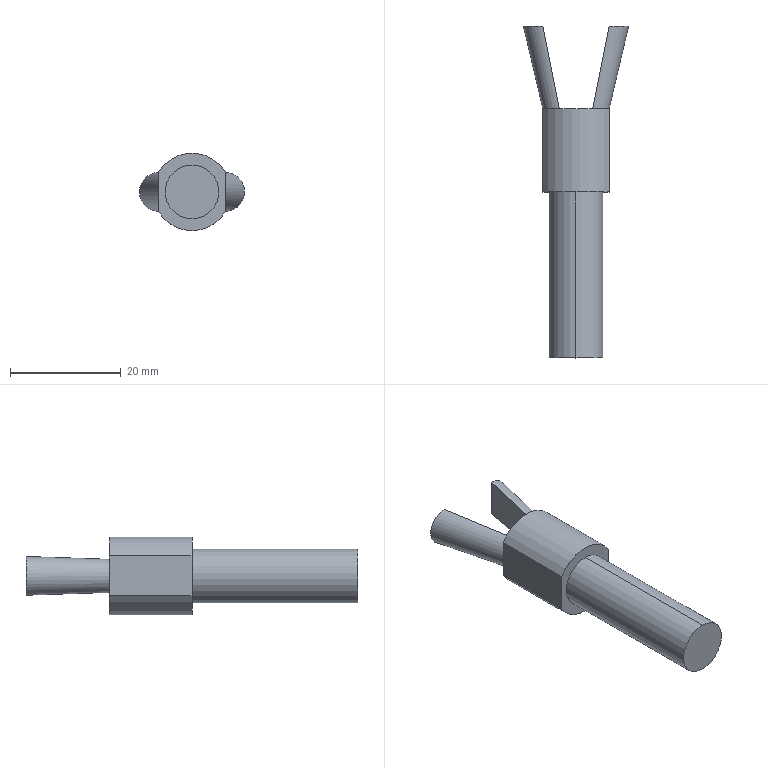Part | 1 solid | 16 faces | box 19 x 60 x 14 mm | volume 4878 mm3 | plane 9 | cylinder 5 | spline 2 | commonest cylinder face diameters 14 x3 9.7 x2
STEP:
#1=CARTESIAN_POINT('',(0.,30.,4.85));
#2=VERTEX_POINT('',#1);
#3=CARTESIAN_POINT('',(0.,30.,-4.85));
#4=VERTEX_POINT('',#3);
#5=CARTESIAN_POINT('',(0.,30.,0.));
#6=DIRECTION('',(0.,1.,0.));
#7=DIRECTION('',(0.,0.,1.));
#8=AXIS2_PLACEMENT_3D('',#5,#6,#7);
#9=CIRCLE('',#8,4.85);
#10=EDGE_CURVE('',#2,#4,#9,.T.);
#11=ORIENTED_EDGE('',*,*,#10,.F.);
#12=CARTESIAN_POINT('',(0.,0.,4.85));
#13=VERTEX_POINT('',#12);
#14=CARTESIAN_POINT('',(0.,30.,4.85));
#15=DIRECTION('',(0.,-1.,0.));
#16=VECTOR('',#15,1000.);
#17=LINE('',#14,#16);
#18=EDGE_CURVE('',#2,#13,#17,.T.);
#19=ORIENTED_EDGE('',*,*,#18,.T.);
#20=CARTESIAN_POINT('',(0.,0.,-4.85));
#21=VERTEX_POINT('',#20);
#22=CARTESIAN_POINT('',(0.,0.,0.));
#23=DIRECTION('',(0.,1.,0.));
#24=DIRECTION('',(0.,0.,1.));
#25=AXIS2_PLACEMENT_3D('',#22,#23,#24);
#26=CIRCLE('',#25,4.85);
#27=EDGE_CURVE('',#13,#21,#26,.T.);
#28=ORIENTED_EDGE('',*,*,#27,.T.);
#29=CARTESIAN_POINT('',(0.,30.,-4.85));
#30=DIRECTION('',(0.,-1.,0.));
#31=VECTOR('',#30,1000.);
#32=LINE('',#29,#31);
#33=EDGE_CURVE('',#4,#21,#32,.T.);
#34=ORIENTED_EDGE('',*,*,#33,.F.);
#35=EDGE_LOOP('',(#11,#19,#28,#34));
#36=FACE_OUTER_BOUND('',#35,.T.);
#37=CARTESIAN_POINT('',(0.,30.,0.));
#38=DIRECTION('',(0.,-1.,0.));
#39=DIRECTION('',(0.,0.,-1.));
#40=AXIS2_PLACEMENT_3D('',#37,#38,#39);
#41=CYLINDRICAL_SURFACE('',#40,4.85);
#42=ADVANCED_FACE('',(#36),#41,.T.);
#43=CARTESIAN_POINT('',(0.,45.,-7.));
#44=VERTEX_POINT('',#43);
#45=CARTESIAN_POINT('',(-6.,45.,-3.606));
#46=VERTEX_POINT('',#45);
#47=CARTESIAN_POINT('',(0.,45.,0.));
#48=DIRECTION('',(0.,1.,0.));
#49=DIRECTION('',(0.,0.,1.));
#50=AXIS2_PLACEMENT_3D('',#47,#48,#49);
#51=CIRCLE('',#50,7.);
#52=EDGE_CURVE('',#44,#46,#51,.T.);
#53=ORIENTED_EDGE('',*,*,#52,.F.);
#54=CARTESIAN_POINT('',(0.,30.,-7.));
#55=VERTEX_POINT('',#54);
#56=CARTESIAN_POINT('',(0.,45.,-7.));
#57=DIRECTION('',(0.,-1.,0.));
#58=VECTOR('',#57,1000.);
#59=LINE('',#56,#58);
#60=EDGE_CURVE('',#44,#55,#59,.T.);
#61=ORIENTED_EDGE('',*,*,#60,.T.);
#62=CARTESIAN_POINT('',(-6.,30.,-3.606));
#63=VERTEX_POINT('',#62);
#64=CARTESIAN_POINT('',(0.,30.,0.));
#65=DIRECTION('',(0.,1.,0.));
#66=DIRECTION('',(0.,0.,1.));
#67=AXIS2_PLACEMENT_3D('',#64,#65,#66);
#68=CIRCLE('',#67,7.);
#69=EDGE_CURVE('',#55,#63,#68,.T.);
#70=ORIENTED_EDGE('',*,*,#69,.T.);
#71=CARTESIAN_POINT('',(-6.,45.,-3.606));
#72=DIRECTION('',(0.,1.,0.));
#73=VECTOR('',#72,1000.);
#74=LINE('',#71,#73);
#75=EDGE_CURVE('',#63,#46,#74,.T.);
#76=ORIENTED_EDGE('',*,*,#75,.T.);
#77=EDGE_LOOP('',(#53,#61,#70,#76));
#78=FACE_OUTER_BOUND('',#77,.T.);
#79=CARTESIAN_POINT('',(0.,45.,0.));
#80=DIRECTION('',(0.,-1.,0.));
#81=DIRECTION('',(0.,0.,-1.));
#82=AXIS2_PLACEMENT_3D('',#79,#80,#81);
#83=CYLINDRICAL_SURFACE('',#82,7.);
#84=ADVANCED_FACE('',(#78),#83,.T.);
#85=CARTESIAN_POINT('',(3.,45.,-3.));
#86=VERTEX_POINT('',#85);
#87=CARTESIAN_POINT('',(3.,45.,3.));
#88=VERTEX_POINT('',#87);
#89=CARTESIAN_POINT('',(3.,45.,-3.));
#90=DIRECTION('',(0.,0.,1.));
#91=VECTOR('',#90,1000.);
#92=LINE('',#89,#91);
#93=EDGE_CURVE('',#86,#88,#92,.T.);
#94=ORIENTED_EDGE('',*,*,#93,.F.);
#95=CARTESIAN_POINT('',(6.,45.,0.0002761));
#96=VERTEX_POINT('',#95);
#97=CARTESIAN_POINT('',(6.,45.,0.0002761));
#98=CARTESIAN_POINT('',(6.,45.,0.0001841));
#99=CARTESIAN_POINT('',(6.,45.,0.00009205));
#100=CARTESIAN_POINT('',(6.,45.,-0.25));
#101=CARTESIAN_POINT('',(5.968,45.,-0.4999));
#102=CARTESIAN_POINT('',(5.847,45.,-0.977));
#103=CARTESIAN_POINT('',(5.758,45.,-1.204));
#104=CARTESIAN_POINT('',(5.536,45.,-1.619));
#105=CARTESIAN_POINT('',(5.404,45.,-1.807));
#106=CARTESIAN_POINT('',(5.116,45.,-2.138));
#107=CARTESIAN_POINT('',(4.96,45.,-2.28));
#108=CARTESIAN_POINT('',(4.48,45.,-2.64));
#109=CARTESIAN_POINT('',(4.147,45.,-2.79));
#110=CARTESIAN_POINT('',(3.533,45.,-2.97));
#111=CARTESIAN_POINT('',(3.25,45.,-3.));
#112=CARTESIAN_POINT('',(3.,45.,-3.));
#113=B_SPLINE_CURVE_WITH_KNOTS('',3,(#97,#98,#99,#100,#101,#102,#103,#104,#105,#106,#107,#108,#109,#110,#111,#112),.UNSPECIFIED.,.F.,.F.,(4,2,2,2,2,2,2,4),(0.,0.000000216,0.0005861,0.001172,0.001758,0.002344,0.003515,0.004687),.UNSPECIFIED.);
#114=EDGE_CURVE('',#96,#86,#113,.T.);
#115=ORIENTED_EDGE('',*,*,#114,.F.);
#116=CARTESIAN_POINT('',(6.,45.,-3.606));
#117=VERTEX_POINT('',#116);
#118=CARTESIAN_POINT('',(6.,45.,-7.));
#119=DIRECTION('',(0.,0.,1.));
#120=VECTOR('',#119,1000.);
#121=LINE('',#118,#120);
#122=EDGE_CURVE('',#117,#96,#121,.T.);
#123=ORIENTED_EDGE('',*,*,#122,.F.);
#124=CARTESIAN_POINT('',(0.,45.,0.));
#125=DIRECTION('',(0.,1.,0.));
#126=DIRECTION('',(0.,0.,1.));
#127=AXIS2_PLACEMENT_3D('',#124,#125,#126);
#128=CIRCLE('',#127,7.);
#129=EDGE_CURVE('',#117,#44,#128,.T.);
#130=ORIENTED_EDGE('',*,*,#129,.T.);
#131=ORIENTED_EDGE('',*,*,#52,.T.);
#132=CARTESIAN_POINT('',(-6.,45.,-0.000828));
#133=VERTEX_POINT('',#132);
#134=CARTESIAN_POINT('',(-6.,45.,-7.));
#135=DIRECTION('',(0.,0.,1.));
#136=VECTOR('',#135,1000.);
#137=LINE('',#134,#136);
#138=EDGE_CURVE('',#46,#133,#137,.T.);
#139=ORIENTED_EDGE('',*,*,#138,.T.);
#140=CARTESIAN_POINT('',(-3.,45.,-3.));
#141=VERTEX_POINT('',#140);
#142=CARTESIAN_POINT('',(-3.,45.,-3.));
#143=CARTESIAN_POINT('',(-3.25,45.,-3.));
#144=CARTESIAN_POINT('',(-3.533,45.,-2.97));
#145=CARTESIAN_POINT('',(-4.147,45.,-2.79));
#146=CARTESIAN_POINT('',(-4.48,45.,-2.64));
#147=CARTESIAN_POINT('',(-4.96,45.,-2.28));
#148=CARTESIAN_POINT('',(-5.116,45.,-2.138));
#149=CARTESIAN_POINT('',(-5.404,45.,-1.807));
#150=CARTESIAN_POINT('',(-5.536,45.,-1.619));
#151=CARTESIAN_POINT('',(-5.758,45.,-1.204));
#152=CARTESIAN_POINT('',(-5.847,45.,-0.977));
#153=CARTESIAN_POINT('',(-5.968,45.,-0.5001));
#154=CARTESIAN_POINT('',(-6.,45.,-0.2506));
#155=CARTESIAN_POINT('',(-6.,45.,-0.000828));
#156=B_SPLINE_CURVE_WITH_KNOTS('',3,(#142,#143,#144,#145,#146,#147,#148,#149,#150,#151,#152,#153,#154,#155),.UNSPECIFIED.,.F.,.F.,(4,2,2,2,2,2,4),(0.,0.125,0.25,0.3125,0.375,0.4375,0.4999),.UNSPECIFIED.);
#157=EDGE_CURVE('',#141,#133,#156,.T.);
#158=ORIENTED_EDGE('',*,*,#157,.F.);
#159=CARTESIAN_POINT('',(-3.,45.,3.));
#160=VERTEX_POINT('',#159);
#161=CARTESIAN_POINT('',(-3.,45.,0.));
#162=DIRECTION('',(0.,0.,-1.));
#163=VECTOR('',#162,1000.);
#164=LINE('',#161,#163);
#165=EDGE_CURVE('',#160,#141,#164,.T.);
#166=ORIENTED_EDGE('',*,*,#165,.F.);
#167=CARTESIAN_POINT('',(-3.,45.,3.));
#168=CARTESIAN_POINT('',(-3.25,45.,3.));
#169=CARTESIAN_POINT('',(-3.533,45.,2.97));
#170=CARTESIAN_POINT('',(-4.147,45.,2.79));
#171=CARTESIAN_POINT('',(-4.48,45.,2.64));
#172=CARTESIAN_POINT('',(-4.96,45.,2.28));
#173=CARTESIAN_POINT('',(-5.116,45.,2.138));
#174=CARTESIAN_POINT('',(-5.404,45.,1.807));
#175=CARTESIAN_POINT('',(-5.536,45.,1.619));
#176=CARTESIAN_POINT('',(-5.758,45.,1.204));
#177=CARTESIAN_POINT('',(-5.847,45.,0.977));
#178=CARTESIAN_POINT('',(-5.968,45.,0.4999));
#179=CARTESIAN_POINT('',(-6.,45.,0.25));
#180=CARTESIAN_POINT('',(-6.,45.,-0.000276));
#181=CARTESIAN_POINT('',(-6.,45.,-0.000552));
#182=CARTESIAN_POINT('',(-6.,45.,-0.000828));
#183=B_SPLINE_CURVE_WITH_KNOTS('',3,(#167,#168,#169,#170,#171,#172,#173,#174,#175,#176,#177,#178,#179,#180,#181,#182),.UNSPECIFIED.,.F.,.F.,(4,2,2,2,2,2,2,4),(0.,0.001172,0.002343,0.002929,0.003515,0.004101,0.004687,0.004687),.UNSPECIFIED.);
#184=EDGE_CURVE('',#160,#133,#183,.T.);
#185=ORIENTED_EDGE('',*,*,#184,.T.);
#186=CARTESIAN_POINT('',(-6.,45.,3.606));
#187=VERTEX_POINT('',#186);
#188=CARTESIAN_POINT('',(-6.,45.,-7.));
#189=DIRECTION('',(0.,0.,1.));
#190=VECTOR('',#189,1000.);
#191=LINE('',#188,#190);
#192=EDGE_CURVE('',#133,#187,#191,.T.);
#193=ORIENTED_EDGE('',*,*,#192,.T.);
#194=CARTESIAN_POINT('',(6.,45.,3.606));
#195=VERTEX_POINT('',#194);
#196=CARTESIAN_POINT('',(0.,45.,0.));
#197=DIRECTION('',(0.,1.,0.));
#198=DIRECTION('',(0.,0.,1.));
#199=AXIS2_PLACEMENT_3D('',#196,#197,#198);
#200=CIRCLE('',#199,7.);
#201=EDGE_CURVE('',#187,#195,#200,.T.);
#202=ORIENTED_EDGE('',*,*,#201,.T.);
#203=CARTESIAN_POINT('',(6.,45.,-7.));
#204=DIRECTION('',(0.,0.,1.));
#205=VECTOR('',#204,1000.);
#206=LINE('',#203,#205);
#207=EDGE_CURVE('',#96,#195,#206,.T.);
#208=ORIENTED_EDGE('',*,*,#207,.F.);
#209=CARTESIAN_POINT('',(3.,45.,3.));
#210=CARTESIAN_POINT('',(3.25,45.,3.));
#211=CARTESIAN_POINT('',(3.533,45.,2.97));
#212=CARTESIAN_POINT('',(4.147,45.,2.79));
#213=CARTESIAN_POINT('',(4.48,45.,2.64));
#214=CARTESIAN_POINT('',(4.96,45.,2.28));
#215=CARTESIAN_POINT('',(5.116,45.,2.138));
#216=CARTESIAN_POINT('',(5.404,45.,1.807));
#217=CARTESIAN_POINT('',(5.536,45.,1.619));
#218=CARTESIAN_POINT('',(5.758,45.,1.204));
#219=CARTESIAN_POINT('',(5.847,45.,0.977));
#220=CARTESIAN_POINT('',(5.968,45.,0.5));
#221=CARTESIAN_POINT('',(6.,45.,0.2502));
#222=CARTESIAN_POINT('',(6.,45.,0.0002761));
#223=B_SPLINE_CURVE_WITH_KNOTS('',3,(#209,#210,#211,#212,#213,#214,#215,#216,#217,#218,#219,#220,#221,#222),.UNSPECIFIED.,.F.,.F.,(4,2,2,2,2,2,4),(0.,0.125,0.25,0.3125,0.375,0.4375,0.5),.UNSPECIFIED.);
#224=EDGE_CURVE('',#88,#96,#223,.T.);
#225=ORIENTED_EDGE('',*,*,#224,.F.);
#226=EDGE_LOOP('',(#94,#115,#123,#130,#131,#139,#158,#166,#185,#193,#202,#208,#225));
#227=FACE_OUTER_BOUND('',#226,.T.);
#228=CARTESIAN_POINT('',(0.,45.,0.));
#229=DIRECTION('',(0.,1.,0.));
#230=DIRECTION('',(0.,0.,1.));
#231=AXIS2_PLACEMENT_3D('',#228,#229,#230);
#232=PLANE('',#231);
#233=ADVANCED_FACE('',(#227),#232,.T.);
#234=ORIENTED_EDGE('',*,*,#60,.F.);
#235=ORIENTED_EDGE('',*,*,#129,.F.);
#236=CARTESIAN_POINT('',(6.,30.,-3.606));
#237=VERTEX_POINT('',#236);
#238=CARTESIAN_POINT('',(6.,45.,-3.606));
#239=DIRECTION('',(0.,-1.,0.));
#240=VECTOR('',#239,1000.);
#241=LINE('',#238,#240);
#242=EDGE_CURVE('',#117,#237,#241,.T.);
#243=ORIENTED_EDGE('',*,*,#242,.T.);
#244=CARTESIAN_POINT('',(0.,30.,0.));
#245=DIRECTION('',(0.,1.,0.));
#246=DIRECTION('',(0.,0.,1.));
#247=AXIS2_PLACEMENT_3D('',#244,#245,#246);
#248=CIRCLE('',#247,7.);
#249=EDGE_CURVE('',#237,#55,#248,.T.);
#250=ORIENTED_EDGE('',*,*,#249,.T.);
#251=EDGE_LOOP('',(#234,#235,#243,#250));
#252=FACE_OUTER_BOUND('',#251,.T.);
#253=CARTESIAN_POINT('',(0.,45.,0.));
#254=DIRECTION('',(0.,-1.,0.));
#255=DIRECTION('',(0.,0.,-1.));
#256=AXIS2_PLACEMENT_3D('',#253,#254,#255);
#257=CYLINDRICAL_SURFACE('',#256,7.);
#258=ADVANCED_FACE('',(#252),#257,.T.);
#259=ORIENTED_EDGE('',*,*,#18,.F.);
#260=CARTESIAN_POINT('',(0.,30.,0.));
#261=DIRECTION('',(0.,1.,0.));
#262=DIRECTION('',(0.,0.,1.));
#263=AXIS2_PLACEMENT_3D('',#260,#261,#262);
#264=CIRCLE('',#263,4.85);
#265=EDGE_CURVE('',#4,#2,#264,.T.);
#266=ORIENTED_EDGE('',*,*,#265,.F.);
#267=ORIENTED_EDGE('',*,*,#33,.T.);
#268=CARTESIAN_POINT('',(0.,0.,0.));
#269=DIRECTION('',(0.,1.,0.));
#270=DIRECTION('',(0.,0.,1.));
#271=AXIS2_PLACEMENT_3D('',#268,#269,#270);
#272=CIRCLE('',#271,4.85);
#273=EDGE_CURVE('',#21,#13,#272,.T.);
#274=ORIENTED_EDGE('',*,*,#273,.T.);
#275=EDGE_LOOP('',(#259,#266,#267,#274));
#276=FACE_OUTER_BOUND('',#275,.T.);
#277=CARTESIAN_POINT('',(0.,30.,0.));
#278=DIRECTION('',(0.,-1.,0.));
#279=DIRECTION('',(0.,0.,-1.));
#280=AXIS2_PLACEMENT_3D('',#277,#278,#279);
#281=CYLINDRICAL_SURFACE('',#280,4.85);
#282=ADVANCED_FACE('',(#276),#281,.T.);
#283=ORIENTED_EDGE('',*,*,#273,.F.);
#284=ORIENTED_EDGE('',*,*,#27,.F.);
#285=EDGE_LOOP('',(#283,#284));
#286=FACE_OUTER_BOUND('',#285,.T.);
#287=CARTESIAN_POINT('',(0.,0.,0.));
#288=DIRECTION('',(0.,1.,0.));
#289=DIRECTION('',(0.,0.,1.));
#290=AXIS2_PLACEMENT_3D('',#287,#288,#289);
#291=PLANE('',#290);
#292=ADVANCED_FACE('',(#286),#291,.F.);
#293=CARTESIAN_POINT('',(-6.,30.,3.606));
#294=VERTEX_POINT('',#293);
#295=CARTESIAN_POINT('',(6.,30.,3.606));
#296=VERTEX_POINT('',#295);
#297=CARTESIAN_POINT('',(0.,30.,0.));
#298=DIRECTION('',(0.,1.,0.));
#299=DIRECTION('',(0.,0.,1.));
#300=AXIS2_PLACEMENT_3D('',#297,#298,#299);
#301=CIRCLE('',#300,7.);
#302=EDGE_CURVE('',#294,#296,#301,.T.);
#303=ORIENTED_EDGE('',*,*,#302,.T.);
#304=CARTESIAN_POINT('',(6.,45.,3.606));
#305=DIRECTION('',(0.,1.,0.));
#306=VECTOR('',#305,1000.);
#307=LINE('',#304,#306);
#308=EDGE_CURVE('',#296,#195,#307,.T.);
#309=ORIENTED_EDGE('',*,*,#308,.T.);
#310=ORIENTED_EDGE('',*,*,#201,.F.);
#311=CARTESIAN_POINT('',(-6.,45.,3.606));
#312=DIRECTION('',(0.,-1.,0.));
#313=VECTOR('',#312,1000.);
#314=LINE('',#311,#313);
#315=EDGE_CURVE('',#187,#294,#314,.T.);
#316=ORIENTED_EDGE('',*,*,#315,.T.);
#317=EDGE_LOOP('',(#303,#309,#310,#316));
#318=FACE_OUTER_BOUND('',#317,.T.);
#319=CARTESIAN_POINT('',(0.,45.,0.));
#320=DIRECTION('',(0.,-1.,0.));
#321=DIRECTION('',(0.,0.,-1.));
#322=AXIS2_PLACEMENT_3D('',#319,#320,#321);
#323=CYLINDRICAL_SURFACE('',#322,7.);
#324=ADVANCED_FACE('',(#318),#323,.T.);
#325=ORIENTED_EDGE('',*,*,#265,.T.);
#326=ORIENTED_EDGE('',*,*,#10,.T.);
#327=EDGE_LOOP('',(#325,#326));
#328=FACE_BOUND('',#327,.T.);
#329=ORIENTED_EDGE('',*,*,#249,.F.);
#330=CARTESIAN_POINT('',(6.,30.,0.));
#331=DIRECTION('',(0.,0.,1.));
#332=VECTOR('',#331,1000.);
#333=LINE('',#330,#332);
#334=EDGE_CURVE('',#237,#296,#333,.T.);
#335=ORIENTED_EDGE('',*,*,#334,.T.);
#336=ORIENTED_EDGE('',*,*,#302,.F.);
#337=CARTESIAN_POINT('',(-6.,30.,0.));
#338=DIRECTION('',(0.,0.,-1.));
#339=VECTOR('',#338,1000.);
#340=LINE('',#337,#339);
#341=EDGE_CURVE('',#294,#63,#340,.T.);
#342=ORIENTED_EDGE('',*,*,#341,.T.);
#343=ORIENTED_EDGE('',*,*,#69,.F.);
#344=EDGE_LOOP('',(#329,#335,#336,#342,#343));
#345=FACE_OUTER_BOUND('',#344,.T.);
#346=CARTESIAN_POINT('',(0.,30.,0.));
#347=DIRECTION('',(0.,1.,0.));
#348=DIRECTION('',(0.,0.,1.));
#349=AXIS2_PLACEMENT_3D('',#346,#347,#348);
#350=PLANE('',#349);
#351=ADVANCED_FACE('',(#328,#345),#350,.F.);
#352=ORIENTED_EDGE('',*,*,#138,.F.);
#353=ORIENTED_EDGE('',*,*,#75,.F.);
#354=ORIENTED_EDGE('',*,*,#341,.F.);
#355=ORIENTED_EDGE('',*,*,#315,.F.);
#356=ORIENTED_EDGE('',*,*,#192,.F.);
#357=EDGE_LOOP('',(#352,#353,#354,#355,#356));
#358=FACE_OUTER_BOUND('',#357,.T.);
#359=CARTESIAN_POINT('',(-6.,45.,-7.));
#360=DIRECTION('',(1.,0.,0.));
#361=DIRECTION('',(0.,1.,0.));
#362=AXIS2_PLACEMENT_3D('',#359,#360,#361);
#363=PLANE('',#362);
#364=ADVANCED_FACE('',(#358),#363,.F.);
#365=ORIENTED_EDGE('',*,*,#122,.T.);
#366=ORIENTED_EDGE('',*,*,#207,.T.);
#367=ORIENTED_EDGE('',*,*,#308,.F.);
#368=ORIENTED_EDGE('',*,*,#334,.F.);
#369=ORIENTED_EDGE('',*,*,#242,.F.);
#370=EDGE_LOOP('',(#365,#366,#367,#368,#369));
#371=FACE_OUTER_BOUND('',#370,.T.);
#372=CARTESIAN_POINT('',(6.,45.,-7.));
#373=DIRECTION('',(-1.,0.,0.));
#374=DIRECTION('',(0.,-1.,0.));
#375=AXIS2_PLACEMENT_3D('',#372,#373,#374);
#376=PLANE('',#375);
#377=ADVANCED_FACE('',(#371),#376,.F.);
#378=CARTESIAN_POINT('',(-6.,60.,-3.5));
#379=VERTEX_POINT('',#378);
#380=CARTESIAN_POINT('',(-6.,60.,3.5));
#381=VERTEX_POINT('',#380);
#382=CARTESIAN_POINT('',(-6.,60.,-3.5));
#383=CARTESIAN_POINT('',(-6.459,60.,-3.5));
#384=CARTESIAN_POINT('',(-6.915,60.,-3.409));
#385=CARTESIAN_POINT('',(-7.763,60.,-3.058));
#386=CARTESIAN_POINT('',(-8.15,60.,-2.799));
#387=CARTESIAN_POINT('',(-8.799,60.,-2.15));
#388=CARTESIAN_POINT('',(-9.058,60.,-1.763));
#389=CARTESIAN_POINT('',(-9.409,60.,-0.9155));
#390=CARTESIAN_POINT('',(-9.5,60.,-0.4589));
#391=CARTESIAN_POINT('',(-9.5,60.,0.4589));
#392=CARTESIAN_POINT('',(-9.409,60.,0.9154));
#393=CARTESIAN_POINT('',(-9.058,60.,1.763));
#394=CARTESIAN_POINT('',(-8.799,60.,2.15));
#395=CARTESIAN_POINT('',(-8.15,60.,2.799));
#396=CARTESIAN_POINT('',(-7.763,60.,3.058));
#397=CARTESIAN_POINT('',(-6.915,60.,3.409));
#398=CARTESIAN_POINT('',(-6.46,60.,3.5));
#399=CARTESIAN_POINT('',(-6.,60.,3.5));
#400=B_SPLINE_CURVE_WITH_KNOTS('',3,(#382,#383,#384,#385,#386,#387,#388,#389,#390,#391,#392,#393,#394,#395,#396,#397,#398,#399),.UNSPECIFIED.,.F.,.F.,(4,2,2,2,2,2,2,2,4),(0.,0.125,0.25,0.375,0.5,0.625,0.75,0.875,1.),.UNSPECIFIED.);
#401=EDGE_CURVE('',#379,#381,#400,.T.);
#402=ORIENTED_EDGE('',*,*,#401,.T.);
#403=CARTESIAN_POINT('',(-6.,60.,3.5));
#404=CARTESIAN_POINT('',(-6.,60.,1.167));
#405=CARTESIAN_POINT('',(-6.,60.,-1.167));
#406=CARTESIAN_POINT('',(-6.,60.,-3.5));
#407=B_SPLINE_CURVE_WITH_KNOTS('',3,(#403,#404,#405,#406),.UNSPECIFIED.,.F.,.F.,(4,4),(0.,1.),.UNSPECIFIED.);
#408=EDGE_CURVE('',#381,#379,#407,.T.);
#409=ORIENTED_EDGE('',*,*,#408,.T.);
#410=EDGE_LOOP('',(#402,#409));
#411=FACE_OUTER_BOUND('',#410,.T.);
#412=CARTESIAN_POINT('',(-6.,60.,0.));
#413=DIRECTION('',(0.,1.,0.));
#414=DIRECTION('',(0.,0.,1.));
#415=AXIS2_PLACEMENT_3D('',#412,#413,#414);
#416=PLANE('',#415);
#417=ADVANCED_FACE('',(#411),#416,.T.);
#418=CARTESIAN_POINT('',(-3.,45.,-3.));
#419=CARTESIAN_POINT('',(-4.,50.,-3.167));
#420=CARTESIAN_POINT('',(-5.,55.,-3.333));
#421=CARTESIAN_POINT('',(-6.,60.,-3.5));
#422=B_SPLINE_CURVE_WITH_KNOTS('',3,(#418,#419,#420,#421),.UNSPECIFIED.,.F.,.F.,(4,4),(0.,1.),.UNSPECIFIED.);
#423=EDGE_CURVE('',#141,#379,#422,.T.);
#424=ORIENTED_EDGE('',*,*,#423,.T.);
#425=ORIENTED_EDGE('',*,*,#408,.F.);
#426=CARTESIAN_POINT('',(-3.,45.,3.));
#427=CARTESIAN_POINT('',(-6.,60.,3.5));
#428=B_SPLINE_CURVE_WITH_KNOTS('',1,(#426,#427),.UNSPECIFIED.,.F.,.F.,(2,2),(0.,1.),.UNSPECIFIED.);
#429=EDGE_CURVE('',#160,#381,#428,.T.);
#430=ORIENTED_EDGE('',*,*,#429,.F.);
#431=ORIENTED_EDGE('',*,*,#165,.T.);
#432=EDGE_LOOP('',(#424,#425,#430,#431));
#433=FACE_OUTER_BOUND('',#432,.T.);
#434=CARTESIAN_POINT('',(5.769,1.154,0.));
#435=DIRECTION('',(-0.9806,-0.1961,0.));
#436=DIRECTION('',(0.1961,-0.9806,0.));
#437=AXIS2_PLACEMENT_3D('',#434,#435,#436);
#438=PLANE('',#437);
#439=ADVANCED_FACE('',(#433),#438,.F.);
#440=ORIENTED_EDGE('',*,*,#157,.T.);
#441=ORIENTED_EDGE('',*,*,#184,.F.);
#442=ORIENTED_EDGE('',*,*,#429,.T.);
#443=ORIENTED_EDGE('',*,*,#401,.F.);
#444=ORIENTED_EDGE('',*,*,#423,.F.);
#445=EDGE_LOOP('',(#440,#441,#442,#443,#444));
#446=FACE_OUTER_BOUND('',#445,.T.);
#447=CARTESIAN_POINT('',(-3.,45.,-3.));
#448=CARTESIAN_POINT('',(-6.,60.,-3.5));
#449=CARTESIAN_POINT('',(-3.25,45.,-3.));
#450=CARTESIAN_POINT('',(-6.292,60.,-3.5));
#451=CARTESIAN_POINT('',(-3.533,45.,-2.97));
#452=CARTESIAN_POINT('',(-6.622,60.,-3.465));
#453=CARTESIAN_POINT('',(-4.147,45.,-2.79));
#454=CARTESIAN_POINT('',(-7.338,60.,-3.255));
#455=CARTESIAN_POINT('',(-4.48,45.,-2.64));
#456=CARTESIAN_POINT('',(-7.727,60.,-3.08));
#457=CARTESIAN_POINT('',(-4.96,45.,-2.28));
#458=CARTESIAN_POINT('',(-8.287,60.,-2.66));
#459=CARTESIAN_POINT('',(-5.116,45.,-2.138));
#460=CARTESIAN_POINT('',(-8.469,60.,-2.494));
#461=CARTESIAN_POINT('',(-5.404,45.,-1.807));
#462=CARTESIAN_POINT('',(-8.805,60.,-2.109));
#463=CARTESIAN_POINT('',(-5.536,45.,-1.619));
#464=CARTESIAN_POINT('',(-8.959,60.,-1.889));
#465=CARTESIAN_POINT('',(-5.758,45.,-1.204));
#466=CARTESIAN_POINT('',(-9.217,60.,-1.405));
#467=CARTESIAN_POINT('',(-5.847,45.,-0.977));
#468=CARTESIAN_POINT('',(-9.322,60.,-1.14));
#469=CARTESIAN_POINT('',(-5.968,45.,-0.4999));
#470=CARTESIAN_POINT('',(-9.463,60.,-0.5832));
#471=CARTESIAN_POINT('',(-6.,45.,-0.25));
#472=CARTESIAN_POINT('',(-9.5,60.,-0.2917));
#473=CARTESIAN_POINT('',(-6.,45.,0.25));
#474=CARTESIAN_POINT('',(-9.5,60.,0.2917));
#475=CARTESIAN_POINT('',(-5.968,45.,0.4999));
#476=CARTESIAN_POINT('',(-9.463,60.,0.5832));
#477=CARTESIAN_POINT('',(-5.847,45.,0.977));
#478=CARTESIAN_POINT('',(-9.322,60.,1.14));
#479=CARTESIAN_POINT('',(-5.758,45.,1.204));
#480=CARTESIAN_POINT('',(-9.217,60.,1.405));
#481=CARTESIAN_POINT('',(-5.536,45.,1.619));
#482=CARTESIAN_POINT('',(-8.959,60.,1.889));
#483=CARTESIAN_POINT('',(-5.404,45.,1.807));
#484=CARTESIAN_POINT('',(-8.805,60.,2.109));
#485=CARTESIAN_POINT('',(-5.116,45.,2.138));
#486=CARTESIAN_POINT('',(-8.469,60.,2.494));
#487=CARTESIAN_POINT('',(-4.96,45.,2.28));
#488=CARTESIAN_POINT('',(-8.287,60.,2.66));
#489=CARTESIAN_POINT('',(-4.48,45.,2.64));
#490=CARTESIAN_POINT('',(-7.727,60.,3.08));
#491=CARTESIAN_POINT('',(-4.147,45.,2.79));
#492=CARTESIAN_POINT('',(-7.338,60.,3.255));
#493=CARTESIAN_POINT('',(-3.533,45.,2.97));
#494=CARTESIAN_POINT('',(-6.622,60.,3.465));
#495=CARTESIAN_POINT('',(-3.25,45.,3.));
#496=CARTESIAN_POINT('',(-6.292,60.,3.5));
#497=CARTESIAN_POINT('',(-3.,45.,3.));
#498=CARTESIAN_POINT('',(-6.,60.,3.5));
#499=B_SPLINE_SURFACE_WITH_KNOTS('',3,1,((#447,#448),(#449,#450),(#451,#452),(#453,#454),(#455,#456),(#457,#458),(#459,#460),(#461,#462),(#463,#464),(#465,#466),(#467,#468),(#469,#470),(#471,#472),(#473,#474),(#475,#476),(#477,#478),(#479,#480),(#481,#482),(#483,#484),(#485,#486),(#487,#488),(#489,#490),(#491,#492),(#493,#494),(#495,#496),(#497,#498)),.UNSPECIFIED.,.F.,.F.,.F.,(4,2,2,2,2,2,2,2,2,2,2,2,4),(2,2),(0.,0.125,0.25,0.3125,0.375,0.4375,0.5,0.5625,0.625,0.6875,0.75,0.875,1.),(0.,1.),.UNSPECIFIED.);
#500=ADVANCED_FACE('',(#446),#499,.T.);
#501=CARTESIAN_POINT('',(6.,60.,3.5));
#502=VERTEX_POINT('',#501);
#503=CARTESIAN_POINT('',(6.,60.,-3.5));
#504=VERTEX_POINT('',#503);
#505=CARTESIAN_POINT('',(6.,60.,3.5));
#506=CARTESIAN_POINT('',(6.459,60.,3.5));
#507=CARTESIAN_POINT('',(6.915,60.,3.409));
#508=CARTESIAN_POINT('',(7.763,60.,3.058));
#509=CARTESIAN_POINT('',(8.15,60.,2.799));
#510=CARTESIAN_POINT('',(8.799,60.,2.15));
#511=CARTESIAN_POINT('',(9.058,60.,1.763));
#512=CARTESIAN_POINT('',(9.409,60.,0.9155));
#513=CARTESIAN_POINT('',(9.5,60.,0.4589));
#514=CARTESIAN_POINT('',(9.5,60.,-0.4589));
#515=CARTESIAN_POINT('',(9.409,60.,-0.9154));
#516=CARTESIAN_POINT('',(9.058,60.,-1.763));
#517=CARTESIAN_POINT('',(8.799,60.,-2.15));
#518=CARTESIAN_POINT('',(8.15,60.,-2.799));
#519=CARTESIAN_POINT('',(7.763,60.,-3.058));
#520=CARTESIAN_POINT('',(6.915,60.,-3.409));
#521=CARTESIAN_POINT('',(6.46,60.,-3.5));
#522=CARTESIAN_POINT('',(6.,60.,-3.5));
#523=B_SPLINE_CURVE_WITH_KNOTS('',3,(#505,#506,#507,#508,#509,#510,#511,#512,#513,#514,#515,#516,#517,#518,#519,#520,#521,#522),.UNSPECIFIED.,.F.,.F.,(4,2,2,2,2,2,2,2,4),(0.,0.125,0.25,0.375,0.5,0.625,0.75,0.875,1.),.UNSPECIFIED.);
#524=EDGE_CURVE('',#502,#504,#523,.T.);
#525=ORIENTED_EDGE('',*,*,#524,.T.);
#526=CARTESIAN_POINT('',(6.,60.,-3.5));
#527=CARTESIAN_POINT('',(6.,60.,-1.167));
#528=CARTESIAN_POINT('',(6.,60.,1.167));
#529=CARTESIAN_POINT('',(6.,60.,3.5));
#530=B_SPLINE_CURVE_WITH_KNOTS('',3,(#526,#527,#528,#529),.UNSPECIFIED.,.F.,.F.,(4,4),(0.,1.),.UNSPECIFIED.);
#531=EDGE_CURVE('',#504,#502,#530,.T.);
#532=ORIENTED_EDGE('',*,*,#531,.T.);
#533=EDGE_LOOP('',(#525,#532));
#534=FACE_OUTER_BOUND('',#533,.T.);
#535=CARTESIAN_POINT('',(6.,60.,0.));
#536=DIRECTION('',(0.,-1.,0.));
#537=DIRECTION('',(0.,0.,-1.));
#538=AXIS2_PLACEMENT_3D('',#535,#536,#537);
#539=PLANE('',#538);
#540=ADVANCED_FACE('',(#534),#539,.F.);
#541=ORIENTED_EDGE('',*,*,#524,.F.);
#542=CARTESIAN_POINT('',(4.5,52.5,3.25));
#543=DIRECTION('',(-0.196,-0.9801,-0.03267));
#544=VECTOR('',#543,1000.);
#545=LINE('',#542,#544);
#546=EDGE_CURVE('',#502,#88,#545,.T.);
#547=ORIENTED_EDGE('',*,*,#546,.T.);
#548=ORIENTED_EDGE('',*,*,#224,.T.);
#549=ORIENTED_EDGE('',*,*,#114,.T.);
#550=CARTESIAN_POINT('',(4.5,52.5,-3.25));
#551=DIRECTION('',(0.196,0.9801,-0.03267));
#552=VECTOR('',#551,1000.);
#553=LINE('',#550,#552);
#554=EDGE_CURVE('',#86,#504,#553,.T.);
#555=ORIENTED_EDGE('',*,*,#554,.T.);
#556=EDGE_LOOP('',(#541,#547,#548,#549,#555));
#557=FACE_OUTER_BOUND('',#556,.T.);
#558=CARTESIAN_POINT('',(6.,60.,-3.5));
#559=CARTESIAN_POINT('',(3.,45.,-3.));
#560=CARTESIAN_POINT('',(6.292,60.,-3.5));
#561=CARTESIAN_POINT('',(3.25,45.,-3.));
#562=CARTESIAN_POINT('',(6.622,60.,-3.465));
#563=CARTESIAN_POINT('',(3.533,45.,-2.97));
#564=CARTESIAN_POINT('',(7.338,60.,-3.255));
#565=CARTESIAN_POINT('',(4.147,45.,-2.79));
#566=CARTESIAN_POINT('',(7.727,60.,-3.08));
#567=CARTESIAN_POINT('',(4.48,45.,-2.64));
#568=CARTESIAN_POINT('',(8.287,60.,-2.66));
#569=CARTESIAN_POINT('',(4.96,45.,-2.28));
#570=CARTESIAN_POINT('',(8.469,60.,-2.494));
#571=CARTESIAN_POINT('',(5.116,45.,-2.138));
#572=CARTESIAN_POINT('',(8.805,60.,-2.109));
#573=CARTESIAN_POINT('',(5.404,45.,-1.807));
#574=CARTESIAN_POINT('',(8.959,60.,-1.889));
#575=CARTESIAN_POINT('',(5.536,45.,-1.619));
#576=CARTESIAN_POINT('',(9.217,60.,-1.405));
#577=CARTESIAN_POINT('',(5.758,45.,-1.204));
#578=CARTESIAN_POINT('',(9.322,60.,-1.14));
#579=CARTESIAN_POINT('',(5.847,45.,-0.977));
#580=CARTESIAN_POINT('',(9.463,60.,-0.5832));
#581=CARTESIAN_POINT('',(5.968,45.,-0.4999));
#582=CARTESIAN_POINT('',(9.5,60.,-0.2917));
#583=CARTESIAN_POINT('',(6.,45.,-0.25));
#584=CARTESIAN_POINT('',(9.5,60.,0.2917));
#585=CARTESIAN_POINT('',(6.,45.,0.25));
#586=CARTESIAN_POINT('',(9.463,60.,0.5832));
#587=CARTESIAN_POINT('',(5.968,45.,0.4999));
#588=CARTESIAN_POINT('',(9.322,60.,1.14));
#589=CARTESIAN_POINT('',(5.847,45.,0.977));
#590=CARTESIAN_POINT('',(9.217,60.,1.405));
#591=CARTESIAN_POINT('',(5.758,45.,1.204));
#592=CARTESIAN_POINT('',(8.959,60.,1.889));
#593=CARTESIAN_POINT('',(5.536,45.,1.619));
#594=CARTESIAN_POINT('',(8.805,60.,2.109));
#595=CARTESIAN_POINT('',(5.404,45.,1.807));
#596=CARTESIAN_POINT('',(8.469,60.,2.494));
#597=CARTESIAN_POINT('',(5.116,45.,2.138));
#598=CARTESIAN_POINT('',(8.287,60.,2.66));
#599=CARTESIAN_POINT('',(4.96,45.,2.28));
#600=CARTESIAN_POINT('',(7.727,60.,3.08));
#601=CARTESIAN_POINT('',(4.48,45.,2.64));
#602=CARTESIAN_POINT('',(7.338,60.,3.255));
#603=CARTESIAN_POINT('',(4.147,45.,2.79));
#604=CARTESIAN_POINT('',(6.622,60.,3.465));
#605=CARTESIAN_POINT('',(3.533,45.,2.97));
#606=CARTESIAN_POINT('',(6.292,60.,3.5));
#607=CARTESIAN_POINT('',(3.25,45.,3.));
#608=CARTESIAN_POINT('',(6.,60.,3.5));
#609=CARTESIAN_POINT('',(3.,45.,3.));
#610=B_SPLINE_SURFACE_WITH_KNOTS('',3,1,((#558,#559),(#560,#561),(#562,#563),(#564,#565),(#566,#567),(#568,#569),(#570,#571),(#572,#573),(#574,#575),(#576,#577),(#578,#579),(#580,#581),(#582,#583),(#584,#585),(#586,#587),(#588,#589),(#590,#591),(#592,#593),(#594,#595),(#596,#597),(#598,#599),(#600,#601),(#602,#603),(#604,#605),(#606,#607),(#608,#609)),.UNSPECIFIED.,.F.,.F.,.F.,(4,2,2,2,2,2,2,2,2,2,2,2,4),(2,2),(0.,0.125,0.25,0.3125,0.375,0.4375,0.5,0.5625,0.625,0.6875,0.75,0.875,1.),(0.,1.),.UNSPECIFIED.);
#611=ADVANCED_FACE('',(#557),#610,.T.);
#612=ORIENTED_EDGE('',*,*,#554,.F.);
#613=ORIENTED_EDGE('',*,*,#93,.T.);
#614=ORIENTED_EDGE('',*,*,#546,.F.);
#615=ORIENTED_EDGE('',*,*,#531,.F.);
#616=EDGE_LOOP('',(#612,#613,#614,#615));
#617=FACE_OUTER_BOUND('',#616,.T.);
#618=CARTESIAN_POINT('',(-5.769,1.154,0.));
#619=DIRECTION('',(-0.9806,0.1961,0.));
#620=DIRECTION('',(-0.1961,-0.9806,0.));
#621=AXIS2_PLACEMENT_3D('',#618,#619,#620);
#622=PLANE('',#621);
#623=ADVANCED_FACE('',(#617),#622,.T.);
#624=CLOSED_SHELL('',(#42,#84,#233,#258,#282,#292,#324,#351,#364,#377,#417,#439,#500,#540,#611,#623));
#625=MANIFOLD_SOLID_BREP('',#624);
#626=CARTESIAN_POINT('',(0.,0.,0.));
#627=DIRECTION('',(0.,0.,1.));
#628=DIRECTION('',(1.,0.,0.));
#629=AXIS2_PLACEMENT_3D('',#626,#627,#628);
#630=(LENGTH_UNIT()NAMED_UNIT(*)SI_UNIT(.MILLI.,.METRE.));
#631=UNCERTAINTY_MEASURE_WITH_UNIT(LENGTH_MEASURE(0.00001),#630,'','');
#632=(NAMED_UNIT(*)PLANE_ANGLE_UNIT()SI_UNIT($,.RADIAN.));
#633=(NAMED_UNIT(*)SI_UNIT($,.STERADIAN.)SOLID_ANGLE_UNIT());
#634=(GEOMETRIC_REPRESENTATION_CONTEXT(3)GLOBAL_UNCERTAINTY_ASSIGNED_CONTEXT((#631))GLOBAL_UNIT_ASSIGNED_CONTEXT((#630,#632,#633))REPRESENTATION_CONTEXT('',''));
#635=ADVANCED_BREP_SHAPE_REPRESENTATION('',(#625,#629),#634);